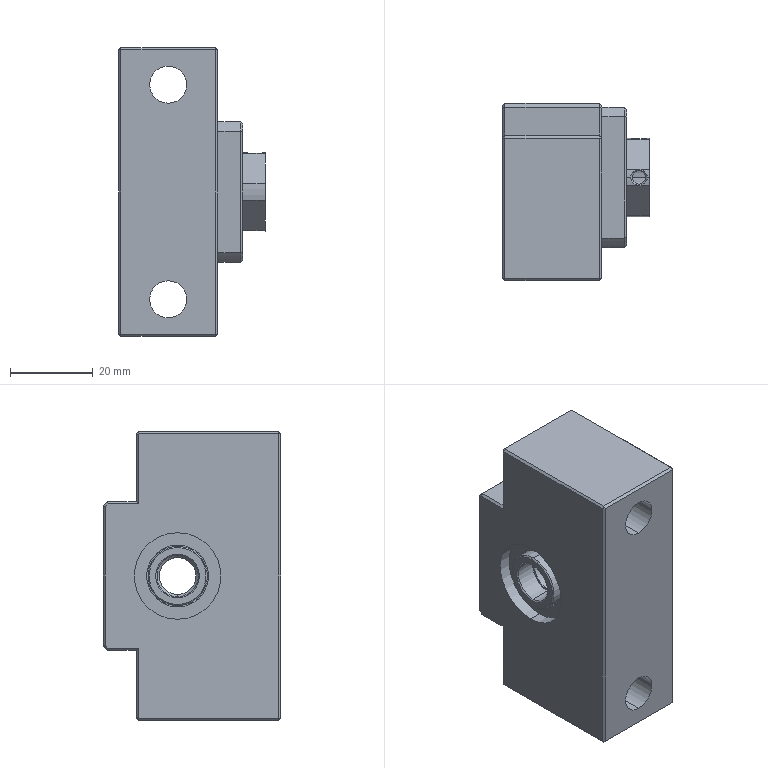Part | SolidWorks | 8 solids | 240 faces | box 35.5 x 43 x 70 mm | volume 61355 mm3 | cylinder 89 | plane 81 | cone 50 | spline 20 | commonest cylinder face diameters 3.242 x12 4.5 x8 8 x8 10 x8 21 x8 14 x6